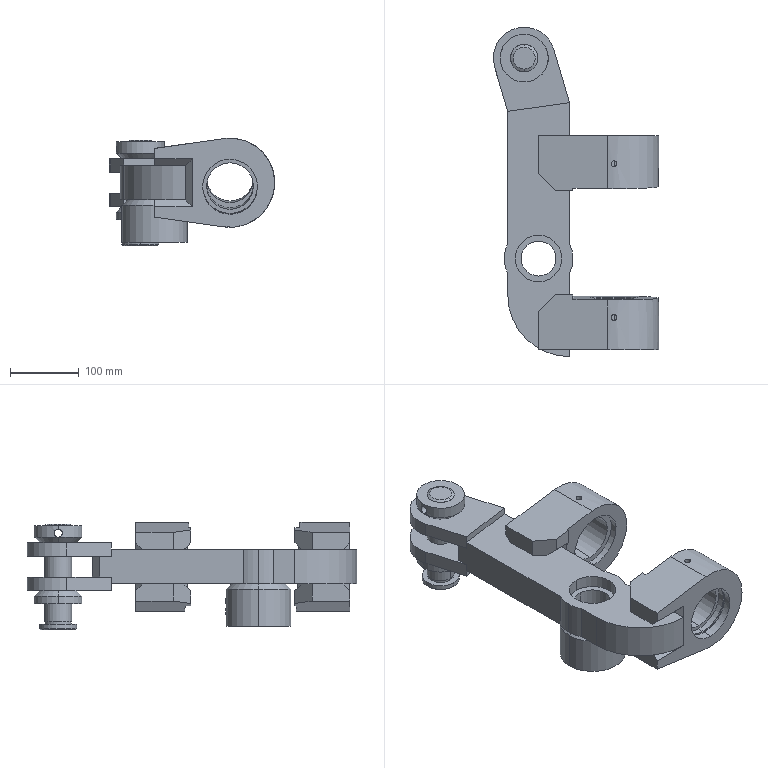Part | SolidWorks | features Cut 2, RefAxis 2, RevCut 2, AEMSimFeature 1 | 9 solids | 165 faces | box 241.001 x 479.989 x 157 mm | volume 4305652 mm3 | plane 83 | cylinder 68 | cone 14 | commonest cylinder face diameters 40 x10 68 x8 80 x8 12 x6 8.5 x4 51 x4